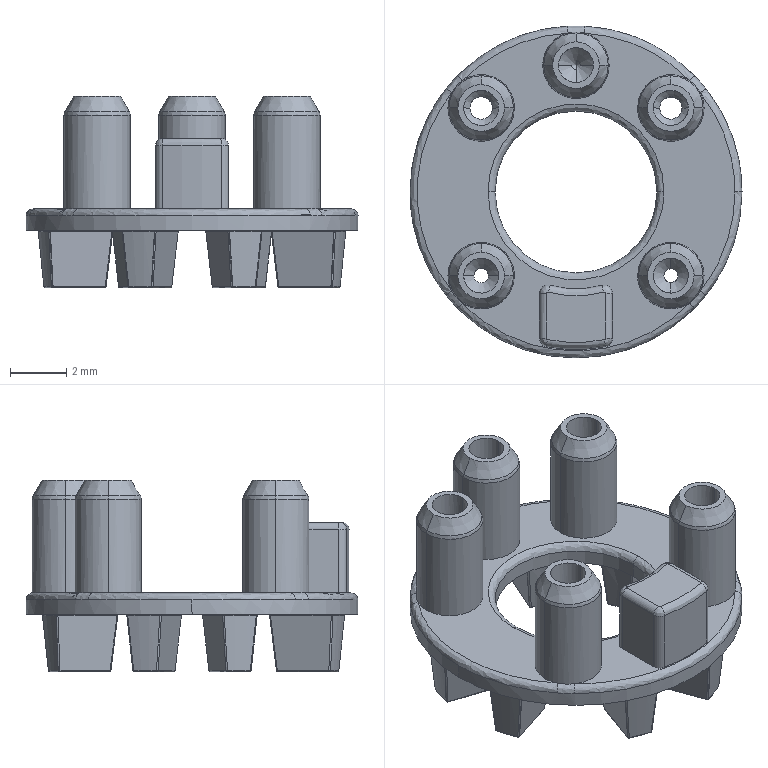Part | STEP file | Product 3 | 1 solid | 352 faces | box 11.8 x 11.8 x 6.802 mm | volume 181.296 mm3 | spline 165 | cylinder 106 | cone 42 | plane 39 | commonest cylinder face diameters 0.102 x56 1.245 x20 2.36 x10 0.6 x4 0.49 x2 0.5 x2